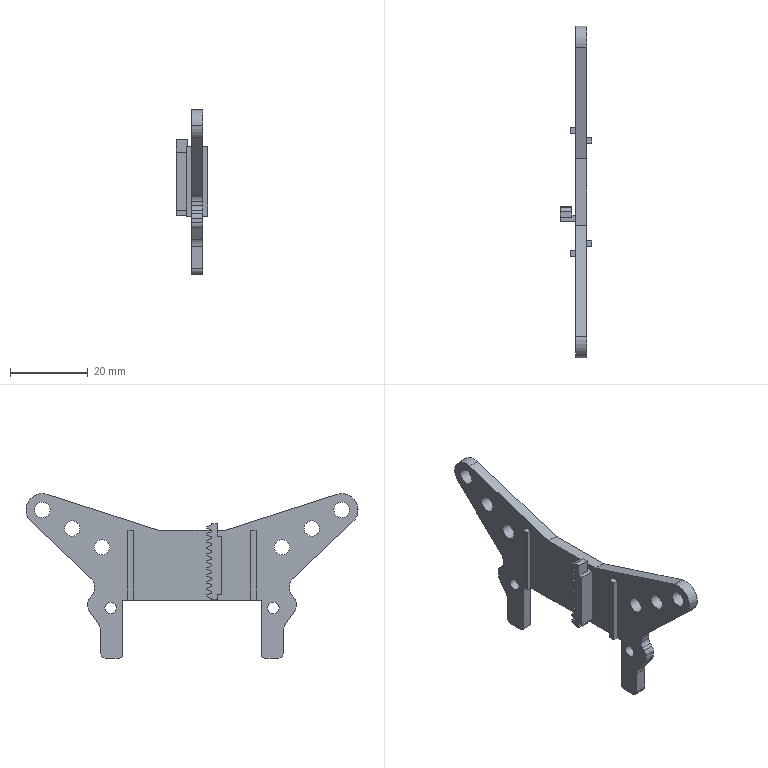Part | STEP file | Dodanie-wyci_gni_cie4_3 | 1 solid | 162 faces | box 8.15 x 85.559 x 42.443 mm | volume 4763 mm3 | plane 93 | cylinder 69 | commonest cylinder face diameters 0.119 x22 0.199 x22 4 x14 3 x6 8.402 x3 6 x2